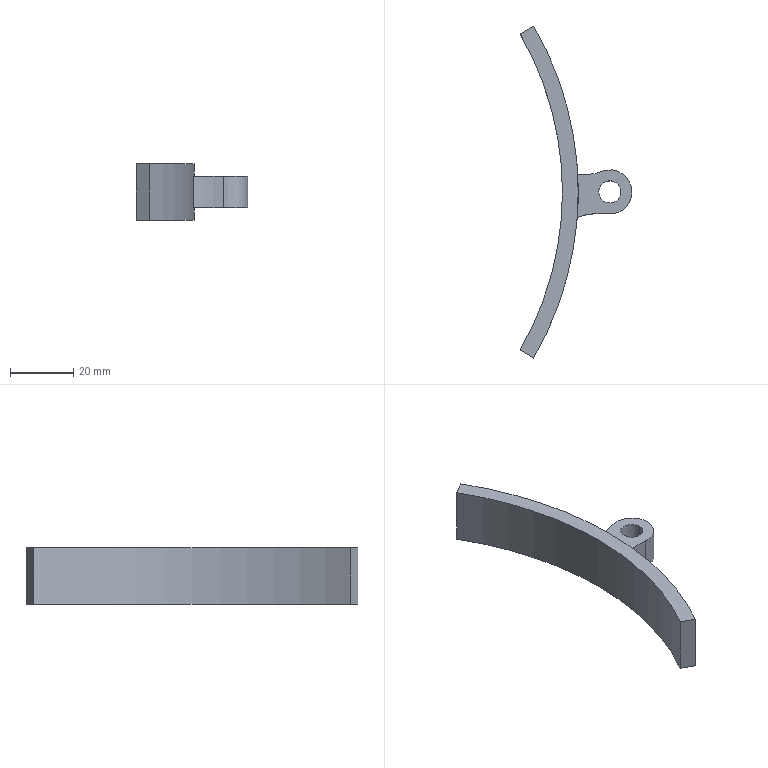Part | SolidWorks | features Extrusion 1, ICE 1 | 1 solid | 13 faces | box 35.397 x 105 x 18 mm | volume 11366 mm3 | cylinder 7 | plane 6 | commonest cylinder face diameters 7 x2 14 x1 30 x1 40 x1 200 x1 210 x1
STEP:
#1=CARTESIAN_POINT('',(111.5,0.,14.));
#2=VERTEX_POINT('',#1);
#3=CARTESIAN_POINT('',(118.5,0.,14.));
#4=VERTEX_POINT('',#3);
#5=CARTESIAN_POINT('',(115.,0.,14.));
#6=DIRECTION('',(0.,0.,1.));
#7=DIRECTION('',(1.,0.,0.));
#8=AXIS2_PLACEMENT_3D('',#5,#6,#7);
#9=CIRCLE('',#8,3.5);
#10=EDGE_CURVE('',#2,#4,#9,.T.);
#11=ORIENTED_EDGE('',*,*,#10,.T.);
#12=CARTESIAN_POINT('',(118.5,0.,4.));
#13=VERTEX_POINT('',#12);
#14=CARTESIAN_POINT('',(118.5,0.,14.));
#15=DIRECTION('',(0.,0.,-1.));
#16=VECTOR('',#15,1000.);
#17=LINE('',#14,#16);
#18=EDGE_CURVE('',#4,#13,#17,.T.);
#19=ORIENTED_EDGE('',*,*,#18,.T.);
#20=CARTESIAN_POINT('',(111.5,0.,4.));
#21=VERTEX_POINT('',#20);
#22=CARTESIAN_POINT('',(115.,0.,4.));
#23=DIRECTION('',(0.,0.,1.));
#24=DIRECTION('',(1.,0.,0.));
#25=AXIS2_PLACEMENT_3D('',#22,#23,#24);
#26=CIRCLE('',#25,3.5);
#27=EDGE_CURVE('',#21,#13,#26,.T.);
#28=ORIENTED_EDGE('',*,*,#27,.F.);
#29=CARTESIAN_POINT('',(111.5,0.,14.));
#30=DIRECTION('',(0.,0.,-1.));
#31=VECTOR('',#30,1000.);
#32=LINE('',#29,#31);
#33=EDGE_CURVE('',#2,#21,#32,.T.);
#34=ORIENTED_EDGE('',*,*,#33,.F.);
#35=EDGE_LOOP('',(#11,#19,#28,#34));
#36=FACE_OUTER_BOUND('',#35,.T.);
#37=CARTESIAN_POINT('',(115.,0.,14.));
#38=DIRECTION('',(0.,0.,-1.));
#39=DIRECTION('',(-1.,0.,0.));
#40=AXIS2_PLACEMENT_3D('',#37,#38,#39);
#41=CYLINDRICAL_SURFACE('',#40,3.5);
#42=ADVANCED_FACE('',(#36),#41,.F.);
#43=CARTESIAN_POINT('',(90.933,-52.5,0.));
#44=VERTEX_POINT('',#43);
#45=CARTESIAN_POINT('',(90.933,52.5,0.));
#46=VERTEX_POINT('',#45);
#47=CARTESIAN_POINT('',(0.,0.,0.));
#48=DIRECTION('',(0.,0.,1.));
#49=DIRECTION('',(1.,0.,0.));
#50=AXIS2_PLACEMENT_3D('',#47,#48,#49);
#51=CIRCLE('',#50,105.);
#52=EDGE_CURVE('',#44,#46,#51,.T.);
#53=ORIENTED_EDGE('',*,*,#52,.T.);
#54=CARTESIAN_POINT('',(90.933,52.5,18.));
#55=VERTEX_POINT('',#54);
#56=CARTESIAN_POINT('',(90.933,52.5,18.));
#57=DIRECTION('',(0.,0.,-1.));
#58=VECTOR('',#57,1000.);
#59=LINE('',#56,#58);
#60=EDGE_CURVE('',#55,#46,#59,.T.);
#61=ORIENTED_EDGE('',*,*,#60,.F.);
#62=CARTESIAN_POINT('',(90.933,-52.5,18.));
#63=VERTEX_POINT('',#62);
#64=CARTESIAN_POINT('',(0.,0.,18.));
#65=DIRECTION('',(0.,0.,1.));
#66=DIRECTION('',(1.,0.,0.));
#67=AXIS2_PLACEMENT_3D('',#64,#65,#66);
#68=CIRCLE('',#67,105.);
#69=EDGE_CURVE('',#63,#55,#68,.T.);
#70=ORIENTED_EDGE('',*,*,#69,.F.);
#71=CARTESIAN_POINT('',(90.933,-52.5,18.));
#72=DIRECTION('',(0.,0.,-1.));
#73=VECTOR('',#72,1000.);
#74=LINE('',#71,#73);
#75=EDGE_CURVE('',#63,#44,#74,.T.);
#76=ORIENTED_EDGE('',*,*,#75,.T.);
#77=EDGE_LOOP('',(#53,#61,#70,#76));
#78=FACE_OUTER_BOUND('',#77,.T.);
#79=CARTESIAN_POINT('',(104.691,-8.053,14.));
#80=VERTEX_POINT('',#79);
#81=CARTESIAN_POINT('',(104.691,-8.053,4.));
#82=VERTEX_POINT('',#81);
#83=CARTESIAN_POINT('',(104.691,-8.053,9.));
#84=DIRECTION('',(0.,0.,-1.));
#85=VECTOR('',#84,1000.);
#86=LINE('',#83,#85);
#87=EDGE_CURVE('',#80,#82,#86,.T.);
#88=ORIENTED_EDGE('',*,*,#87,.F.);
#89=CARTESIAN_POINT('',(104.85,5.618,14.));
#90=VERTEX_POINT('',#89);
#91=CARTESIAN_POINT('',(0.,0.,14.));
#92=DIRECTION('',(0.,0.,1.));
#93=DIRECTION('',(1.,0.,0.));
#94=AXIS2_PLACEMENT_3D('',#91,#92,#93);
#95=CIRCLE('',#94,105.);
#96=EDGE_CURVE('',#80,#90,#95,.T.);
#97=ORIENTED_EDGE('',*,*,#96,.T.);
#98=CARTESIAN_POINT('',(104.85,5.618,4.));
#99=VERTEX_POINT('',#98);
#100=CARTESIAN_POINT('',(104.85,5.618,9.));
#101=DIRECTION('',(0.,0.,1.));
#102=VECTOR('',#101,1000.);
#103=LINE('',#100,#102);
#104=EDGE_CURVE('',#99,#90,#103,.T.);
#105=ORIENTED_EDGE('',*,*,#104,.F.);
#106=CARTESIAN_POINT('',(0.,0.,4.));
#107=DIRECTION('',(0.,0.,1.));
#108=DIRECTION('',(1.,0.,0.));
#109=AXIS2_PLACEMENT_3D('',#106,#107,#108);
#110=CIRCLE('',#109,105.);
#111=EDGE_CURVE('',#82,#99,#110,.T.);
#112=ORIENTED_EDGE('',*,*,#111,.F.);
#113=EDGE_LOOP('',(#88,#97,#105,#112));
#114=FACE_BOUND('',#113,.T.);
#115=CARTESIAN_POINT('',(0.,0.,18.));
#116=DIRECTION('',(0.,0.,-1.));
#117=DIRECTION('',(-1.,0.,0.));
#118=AXIS2_PLACEMENT_3D('',#115,#116,#117);
#119=CYLINDRICAL_SURFACE('',#118,105.);
#120=ADVANCED_FACE('',(#78,#114),#119,.T.);
#121=CARTESIAN_POINT('',(86.603,-50.,0.));
#122=VERTEX_POINT('',#121);
#123=CARTESIAN_POINT('',(86.603,50.,0.));
#124=VERTEX_POINT('',#123);
#125=CARTESIAN_POINT('',(0.,0.,0.));
#126=DIRECTION('',(0.,0.,1.));
#127=DIRECTION('',(1.,0.,0.));
#128=AXIS2_PLACEMENT_3D('',#125,#126,#127);
#129=CIRCLE('',#128,100.);
#130=EDGE_CURVE('',#122,#124,#129,.T.);
#131=ORIENTED_EDGE('',*,*,#130,.F.);
#132=CARTESIAN_POINT('',(86.603,-50.,18.));
#133=VERTEX_POINT('',#132);
#134=CARTESIAN_POINT('',(86.603,-50.,18.));
#135=DIRECTION('',(0.,0.,-1.));
#136=VECTOR('',#135,1000.);
#137=LINE('',#134,#136);
#138=EDGE_CURVE('',#133,#122,#137,.T.);
#139=ORIENTED_EDGE('',*,*,#138,.F.);
#140=CARTESIAN_POINT('',(86.603,50.,18.));
#141=VERTEX_POINT('',#140);
#142=CARTESIAN_POINT('',(0.,0.,18.));
#143=DIRECTION('',(0.,0.,1.));
#144=DIRECTION('',(1.,0.,0.));
#145=AXIS2_PLACEMENT_3D('',#142,#143,#144);
#146=CIRCLE('',#145,100.);
#147=EDGE_CURVE('',#133,#141,#146,.T.);
#148=ORIENTED_EDGE('',*,*,#147,.T.);
#149=CARTESIAN_POINT('',(86.603,50.,18.));
#150=DIRECTION('',(0.,0.,-1.));
#151=VECTOR('',#150,1000.);
#152=LINE('',#149,#151);
#153=EDGE_CURVE('',#141,#124,#152,.T.);
#154=ORIENTED_EDGE('',*,*,#153,.T.);
#155=EDGE_LOOP('',(#131,#139,#148,#154));
#156=FACE_OUTER_BOUND('',#155,.T.);
#157=CARTESIAN_POINT('',(0.,0.,18.));
#158=DIRECTION('',(0.,0.,-1.));
#159=DIRECTION('',(-1.,0.,0.));
#160=AXIS2_PLACEMENT_3D('',#157,#158,#159);
#161=CYLINDRICAL_SURFACE('',#160,100.);
#162=ADVANCED_FACE('',(#156),#161,.F.);
#163=CARTESIAN_POINT('',(86.603,-50.,0.));
#164=DIRECTION('',(0.866,-0.5,0.));
#165=VECTOR('',#164,1000.);
#166=LINE('',#163,#165);
#167=EDGE_CURVE('',#122,#44,#166,.T.);
#168=ORIENTED_EDGE('',*,*,#167,.T.);
#169=ORIENTED_EDGE('',*,*,#75,.F.);
#170=CARTESIAN_POINT('',(86.603,-50.,18.));
#171=DIRECTION('',(0.866,-0.5,0.));
#172=VECTOR('',#171,1000.);
#173=LINE('',#170,#172);
#174=EDGE_CURVE('',#133,#63,#173,.T.);
#175=ORIENTED_EDGE('',*,*,#174,.F.);
#176=ORIENTED_EDGE('',*,*,#138,.T.);
#177=EDGE_LOOP('',(#168,#169,#175,#176));
#178=FACE_OUTER_BOUND('',#177,.T.);
#179=CARTESIAN_POINT('',(86.603,-50.,18.));
#180=DIRECTION('',(0.5,0.866,0.));
#181=DIRECTION('',(-0.866,0.5,0.));
#182=AXIS2_PLACEMENT_3D('',#179,#180,#181);
#183=PLANE('',#182);
#184=ADVANCED_FACE('',(#178),#183,.F.);
#185=CARTESIAN_POINT('',(86.603,50.,0.));
#186=DIRECTION('',(0.866,0.5,0.));
#187=VECTOR('',#186,1000.);
#188=LINE('',#185,#187);
#189=EDGE_CURVE('',#124,#46,#188,.T.);
#190=ORIENTED_EDGE('',*,*,#189,.F.);
#191=ORIENTED_EDGE('',*,*,#153,.F.);
#192=CARTESIAN_POINT('',(86.603,50.,18.));
#193=DIRECTION('',(0.866,0.5,0.));
#194=VECTOR('',#193,1000.);
#195=LINE('',#192,#194);
#196=EDGE_CURVE('',#141,#55,#195,.T.);
#197=ORIENTED_EDGE('',*,*,#196,.T.);
#198=ORIENTED_EDGE('',*,*,#60,.T.);
#199=EDGE_LOOP('',(#190,#191,#197,#198));
#200=FACE_OUTER_BOUND('',#199,.T.);
#201=CARTESIAN_POINT('',(86.603,50.,18.));
#202=DIRECTION('',(-0.5,0.866,0.));
#203=DIRECTION('',(-0.866,-0.5,0.));
#204=AXIS2_PLACEMENT_3D('',#201,#202,#203);
#205=PLANE('',#204);
#206=ADVANCED_FACE('',(#200),#205,.T.);
#207=ORIENTED_EDGE('',*,*,#147,.F.);
#208=ORIENTED_EDGE('',*,*,#174,.T.);
#209=ORIENTED_EDGE('',*,*,#69,.T.);
#210=ORIENTED_EDGE('',*,*,#196,.F.);
#211=EDGE_LOOP('',(#207,#208,#209,#210));
#212=FACE_OUTER_BOUND('',#211,.T.);
#213=CARTESIAN_POINT('',(0.,0.,18.));
#214=DIRECTION('',(0.,0.,1.));
#215=DIRECTION('',(1.,0.,0.));
#216=AXIS2_PLACEMENT_3D('',#213,#214,#215);
#217=PLANE('',#216);
#218=ADVANCED_FACE('',(#212),#217,.T.);
#219=ORIENTED_EDGE('',*,*,#130,.T.);
#220=ORIENTED_EDGE('',*,*,#189,.T.);
#221=ORIENTED_EDGE('',*,*,#52,.F.);
#222=ORIENTED_EDGE('',*,*,#167,.F.);
#223=EDGE_LOOP('',(#219,#220,#221,#222));
#224=FACE_OUTER_BOUND('',#223,.T.);
#225=CARTESIAN_POINT('',(0.,0.,0.));
#226=DIRECTION('',(0.,0.,1.));
#227=DIRECTION('',(1.,0.,0.));
#228=AXIS2_PLACEMENT_3D('',#225,#226,#227);
#229=PLANE('',#228);
#230=ADVANCED_FACE('',(#224),#229,.F.);
#231=CARTESIAN_POINT('',(114.138,-6.947,14.));
#232=VERTEX_POINT('',#231);
#233=CARTESIAN_POINT('',(111.674,-26.794,14.));
#234=DIRECTION('',(0.,0.,-1.));
#235=DIRECTION('',(1.,0.,0.));
#236=AXIS2_PLACEMENT_3D('',#233,#234,#235);
#237=CIRCLE('',#236,20.);
#238=EDGE_CURVE('',#80,#232,#237,.T.);
#239=ORIENTED_EDGE('',*,*,#238,.F.);
#240=ORIENTED_EDGE('',*,*,#87,.T.);
#241=CARTESIAN_POINT('',(114.138,-6.947,4.));
#242=VERTEX_POINT('',#241);
#243=CARTESIAN_POINT('',(111.674,-26.794,4.));
#244=DIRECTION('',(0.,0.,-1.));
#245=DIRECTION('',(1.,0.,0.));
#246=AXIS2_PLACEMENT_3D('',#243,#244,#245);
#247=CIRCLE('',#246,20.);
#248=EDGE_CURVE('',#82,#242,#247,.T.);
#249=ORIENTED_EDGE('',*,*,#248,.T.);
#250=CARTESIAN_POINT('',(114.138,-6.947,14.));
#251=DIRECTION('',(0.,0.,-1.));
#252=VECTOR('',#251,1000.);
#253=LINE('',#250,#252);
#254=EDGE_CURVE('',#232,#242,#253,.T.);
#255=ORIENTED_EDGE('',*,*,#254,.F.);
#256=EDGE_LOOP('',(#239,#240,#249,#255));
#257=FACE_OUTER_BOUND('',#256,.T.);
#258=CARTESIAN_POINT('',(111.674,-26.794,14.));
#259=DIRECTION('',(0.,0.,-1.));
#260=DIRECTION('',(-1.,0.,0.));
#261=AXIS2_PLACEMENT_3D('',#258,#259,#260);
#262=CYLINDRICAL_SURFACE('',#261,20.);
#263=ADVANCED_FACE('',(#257),#262,.F.);
#264=CARTESIAN_POINT('',(112.436,6.514,4.));
#265=VERTEX_POINT('',#264);
#266=CARTESIAN_POINT('',(106.942,20.471,4.));
#267=DIRECTION('',(0.,0.,-1.));
#268=DIRECTION('',(1.,0.,0.));
#269=AXIS2_PLACEMENT_3D('',#266,#267,#268);
#270=CIRCLE('',#269,15.);
#271=EDGE_CURVE('',#265,#99,#270,.T.);
#272=ORIENTED_EDGE('',*,*,#271,.T.);
#273=ORIENTED_EDGE('',*,*,#104,.T.);
#274=CARTESIAN_POINT('',(112.436,6.514,14.));
#275=VERTEX_POINT('',#274);
#276=CARTESIAN_POINT('',(106.942,20.471,14.));
#277=DIRECTION('',(0.,0.,-1.));
#278=DIRECTION('',(1.,0.,0.));
#279=AXIS2_PLACEMENT_3D('',#276,#277,#278);
#280=CIRCLE('',#279,15.);
#281=EDGE_CURVE('',#275,#90,#280,.T.);
#282=ORIENTED_EDGE('',*,*,#281,.F.);
#283=CARTESIAN_POINT('',(112.436,6.514,14.));
#284=DIRECTION('',(0.,0.,-1.));
#285=VECTOR('',#284,1000.);
#286=LINE('',#283,#285);
#287=EDGE_CURVE('',#275,#265,#286,.T.);
#288=ORIENTED_EDGE('',*,*,#287,.T.);
#289=EDGE_LOOP('',(#272,#273,#282,#288));
#290=FACE_OUTER_BOUND('',#289,.T.);
#291=CARTESIAN_POINT('',(106.942,20.471,14.));
#292=DIRECTION('',(0.,0.,-1.));
#293=DIRECTION('',(-1.,0.,0.));
#294=AXIS2_PLACEMENT_3D('',#291,#292,#293);
#295=CYLINDRICAL_SURFACE('',#294,15.);
#296=ADVANCED_FACE('',(#290),#295,.F.);
#297=ORIENTED_EDGE('',*,*,#96,.F.);
#298=ORIENTED_EDGE('',*,*,#238,.T.);
#299=CARTESIAN_POINT('',(115.,0.,14.));
#300=DIRECTION('',(0.,0.,1.));
#301=DIRECTION('',(1.,0.,0.));
#302=AXIS2_PLACEMENT_3D('',#299,#300,#301);
#303=CIRCLE('',#302,7.);
#304=EDGE_CURVE('',#232,#275,#303,.T.);
#305=ORIENTED_EDGE('',*,*,#304,.T.);
#306=ORIENTED_EDGE('',*,*,#281,.T.);
#307=EDGE_LOOP('',(#297,#298,#305,#306));
#308=FACE_OUTER_BOUND('',#307,.T.);
#309=ORIENTED_EDGE('',*,*,#10,.F.);
#310=CARTESIAN_POINT('',(115.,0.,14.));
#311=DIRECTION('',(0.,0.,1.));
#312=DIRECTION('',(1.,0.,0.));
#313=AXIS2_PLACEMENT_3D('',#310,#311,#312);
#314=CIRCLE('',#313,3.5);
#315=EDGE_CURVE('',#4,#2,#314,.T.);
#316=ORIENTED_EDGE('',*,*,#315,.F.);
#317=EDGE_LOOP('',(#309,#316));
#318=FACE_BOUND('',#317,.T.);
#319=CARTESIAN_POINT('',(111.674,-26.794,14.));
#320=DIRECTION('',(0.,0.,1.));
#321=DIRECTION('',(1.,0.,0.));
#322=AXIS2_PLACEMENT_3D('',#319,#320,#321);
#323=PLANE('',#322);
#324=ADVANCED_FACE('',(#308,#318),#323,.T.);
#325=ORIENTED_EDGE('',*,*,#248,.F.);
#326=ORIENTED_EDGE('',*,*,#111,.T.);
#327=ORIENTED_EDGE('',*,*,#271,.F.);
#328=CARTESIAN_POINT('',(115.,0.,4.));
#329=DIRECTION('',(0.,0.,1.));
#330=DIRECTION('',(1.,0.,0.));
#331=AXIS2_PLACEMENT_3D('',#328,#329,#330);
#332=CIRCLE('',#331,7.);
#333=EDGE_CURVE('',#242,#265,#332,.T.);
#334=ORIENTED_EDGE('',*,*,#333,.F.);
#335=EDGE_LOOP('',(#325,#326,#327,#334));
#336=FACE_OUTER_BOUND('',#335,.T.);
#337=ORIENTED_EDGE('',*,*,#27,.T.);
#338=CARTESIAN_POINT('',(115.,0.,4.));
#339=DIRECTION('',(0.,0.,1.));
#340=DIRECTION('',(1.,0.,0.));
#341=AXIS2_PLACEMENT_3D('',#338,#339,#340);
#342=CIRCLE('',#341,3.5);
#343=EDGE_CURVE('',#13,#21,#342,.T.);
#344=ORIENTED_EDGE('',*,*,#343,.T.);
#345=EDGE_LOOP('',(#337,#344));
#346=FACE_BOUND('',#345,.T.);
#347=CARTESIAN_POINT('',(111.674,-26.794,4.));
#348=DIRECTION('',(0.,0.,1.));
#349=DIRECTION('',(1.,0.,0.));
#350=AXIS2_PLACEMENT_3D('',#347,#348,#349);
#351=PLANE('',#350);
#352=ADVANCED_FACE('',(#336,#346),#351,.F.);
#353=ORIENTED_EDGE('',*,*,#333,.T.);
#354=ORIENTED_EDGE('',*,*,#287,.F.);
#355=ORIENTED_EDGE('',*,*,#304,.F.);
#356=ORIENTED_EDGE('',*,*,#254,.T.);
#357=EDGE_LOOP('',(#353,#354,#355,#356));
#358=FACE_OUTER_BOUND('',#357,.T.);
#359=CARTESIAN_POINT('',(115.,0.,14.));
#360=DIRECTION('',(0.,0.,-1.));
#361=DIRECTION('',(-1.,0.,0.));
#362=AXIS2_PLACEMENT_3D('',#359,#360,#361);
#363=CYLINDRICAL_SURFACE('',#362,7.);
#364=ADVANCED_FACE('',(#358),#363,.T.);
#365=ORIENTED_EDGE('',*,*,#18,.F.);
#366=ORIENTED_EDGE('',*,*,#315,.T.);
#367=ORIENTED_EDGE('',*,*,#33,.T.);
#368=ORIENTED_EDGE('',*,*,#343,.F.);
#369=EDGE_LOOP('',(#365,#366,#367,#368));
#370=FACE_OUTER_BOUND('',#369,.T.);
#371=CARTESIAN_POINT('',(115.,0.,14.));
#372=DIRECTION('',(0.,0.,-1.));
#373=DIRECTION('',(-1.,0.,0.));
#374=AXIS2_PLACEMENT_3D('',#371,#372,#373);
#375=CYLINDRICAL_SURFACE('',#374,3.5);
#376=ADVANCED_FACE('',(#370),#375,.F.);
#377=CLOSED_SHELL('',(#42,#120,#162,#184,#206,#218,#230,#263,#296,#324,#352,#364,#376));
#378=MANIFOLD_SOLID_BREP('',#377);
#379=CARTESIAN_POINT('',(0.,0.,0.));
#380=DIRECTION('',(0.,0.,1.));
#381=DIRECTION('',(1.,0.,0.));
#382=AXIS2_PLACEMENT_3D('',#379,#380,#381);
#383=(LENGTH_UNIT()NAMED_UNIT(*)SI_UNIT(.MILLI.,.METRE.));
#384=UNCERTAINTY_MEASURE_WITH_UNIT(LENGTH_MEASURE(0.00001),#383,'','');
#385=(NAMED_UNIT(*)PLANE_ANGLE_UNIT()SI_UNIT($,.RADIAN.));
#386=(NAMED_UNIT(*)SI_UNIT($,.STERADIAN.)SOLID_ANGLE_UNIT());
#387=(GEOMETRIC_REPRESENTATION_CONTEXT(3)GLOBAL_UNCERTAINTY_ASSIGNED_CONTEXT((#384))GLOBAL_UNIT_ASSIGNED_CONTEXT((#383,#385,#386))REPRESENTATION_CONTEXT('',''));
#388=ADVANCED_BREP_SHAPE_REPRESENTATION('',(#378,#382),#387);